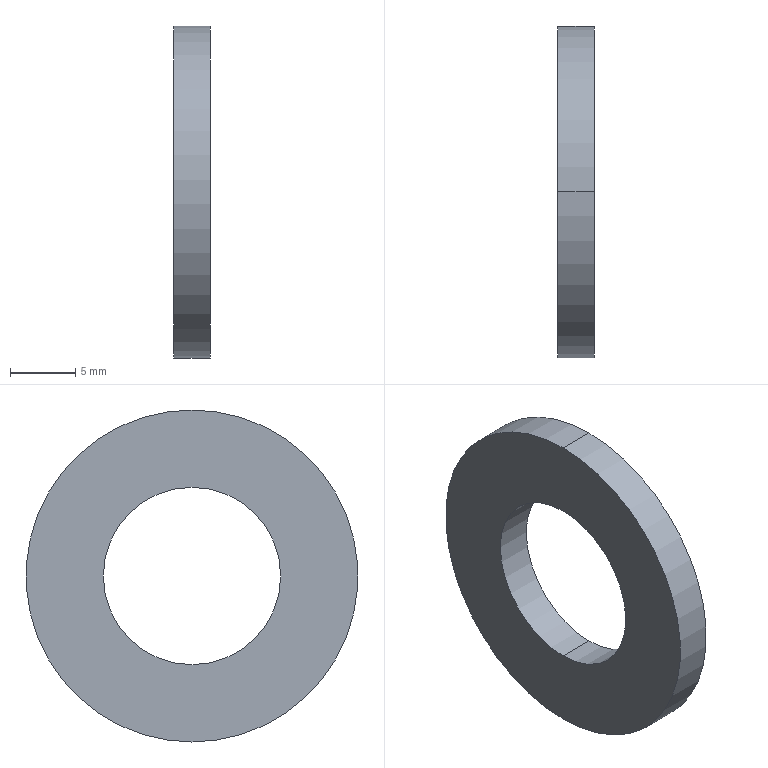Part | STEP file | flat washer narrow_am_B18.22M - Plain washer, 12 mm, narrow | 1 solid | 6 faces | box 2.8 x 25.4 x 25.4 mm | volume 1014 mm3 | cylinder 4 | plane 2 | commonest cylinder face diameters 13.57 x2 25.4 x2
STEP:
#1=CARTESIAN_POINT('',(0.,0.,0.));
#2=DIRECTION('',(0.,0.,1.));
#3=DIRECTION('',(1.,0.,0.));
#4=AXIS2_PLACEMENT_3D('',#1,#2,#3);
#5=CARTESIAN_POINT('',(0.,0.,12.7));
#6=VERTEX_POINT('',#5);
#7=CARTESIAN_POINT('',(0.,0.,-12.7));
#8=VERTEX_POINT('',#7);
#9=CARTESIAN_POINT('',(0.,0.,0.));
#10=DIRECTION('',(-1.,0.,0.));
#11=DIRECTION('',(0.,0.,1.));
#12=AXIS2_PLACEMENT_3D('',#9,#10,#11);
#13=CIRCLE('',#12,12.7);
#14=CARTESIAN_POINT('',(-34.925,0.,0.));
#15=DIRECTION('',(-1.,0.,0.));
#16=DIRECTION('',(0.,0.,1.));
#17=AXIS2_PLACEMENT_3D('',#14,#15,#16);
#18=CYLINDRICAL_SURFACE('',#17,12.7);
#19=CARTESIAN_POINT('',(0.,-34.925));
#20=DIRECTION('',(1.,0.));
#21=VECTOR('',#20,1.);
#22=LINE('',#19,#21);
#23=(GEOMETRIC_REPRESENTATION_CONTEXT(2)PARAMETRIC_REPRESENTATION_CONTEXT()REPRESENTATION_CONTEXT('',''));
#24=DEFINITIONAL_REPRESENTATION('',(#22),#23);
#25=PCURVE('',#18,#24);
#26=CARTESIAN_POINT('',(0.,6.785,0.));
#27=DIRECTION('',(-1.,0.,0.));
#28=DIRECTION('',(0.,0.,1.));
#29=AXIS2_PLACEMENT_3D('',#26,#27,#28);
#30=PLANE('',#29);
#31=CARTESIAN_POINT('',(0.,-6.785));
#32=DIRECTION('',(1.,0.));
#33=AXIS2_PLACEMENT_2D('',#31,#32);
#34=CIRCLE('',#33,12.7);
#35=(GEOMETRIC_REPRESENTATION_CONTEXT(2)PARAMETRIC_REPRESENTATION_CONTEXT()REPRESENTATION_CONTEXT('',''));
#36=DEFINITIONAL_REPRESENTATION('',(#34),#35);
#37=PCURVE('',#30,#36);
#38=SURFACE_CURVE('',#13,(#25,#37),.PCURVE_S1.);
#39=EDGE_CURVE('',#6,#8,#38,.T.);
#40=ORIENTED_EDGE('',*,*,#39,.T.);
#41=CARTESIAN_POINT('',(-2.8,0.,-12.7));
#42=VERTEX_POINT('',#41);
#43=CARTESIAN_POINT('',(-34.925,0.,-12.7));
#44=DIRECTION('',(-1.,0.,0.));
#45=VECTOR('',#44,1.);
#46=LINE('',#43,#45);
#47=CARTESIAN_POINT('',(3.142,0.));
#48=DIRECTION('',(0.,1.));
#49=VECTOR('',#48,1.);
#50=LINE('',#47,#49);
#51=(GEOMETRIC_REPRESENTATION_CONTEXT(2)PARAMETRIC_REPRESENTATION_CONTEXT()REPRESENTATION_CONTEXT('',''));
#52=DEFINITIONAL_REPRESENTATION('',(#50),#51);
#53=PCURVE('',#18,#52);
#54=CARTESIAN_POINT('',(-34.925,0.,0.));
#55=DIRECTION('',(-1.,0.,0.));
#56=DIRECTION('',(0.,0.,1.));
#57=AXIS2_PLACEMENT_3D('',#54,#55,#56);
#58=CYLINDRICAL_SURFACE('',#57,12.7);
#59=CARTESIAN_POINT('',(3.142,0.));
#60=DIRECTION('',(0.,1.));
#61=VECTOR('',#60,1.);
#62=LINE('',#59,#61);
#63=(GEOMETRIC_REPRESENTATION_CONTEXT(2)PARAMETRIC_REPRESENTATION_CONTEXT()REPRESENTATION_CONTEXT('',''));
#64=DEFINITIONAL_REPRESENTATION('',(#62),#63);
#65=PCURVE('',#58,#64);
#66=SURFACE_CURVE('',#46,(#53,#65),.PCURVE_S1.);
#67=EDGE_CURVE('',#8,#42,#66,.T.);
#68=ORIENTED_EDGE('',*,*,#67,.T.);
#69=CARTESIAN_POINT('',(-2.8,0.,12.7));
#70=VERTEX_POINT('',#69);
#71=CARTESIAN_POINT('',(-2.8,0.,0.));
#72=DIRECTION('',(-1.,0.,0.));
#73=DIRECTION('',(0.,0.,1.));
#74=AXIS2_PLACEMENT_3D('',#71,#72,#73);
#75=CIRCLE('',#74,12.7);
#76=CARTESIAN_POINT('',(0.,-32.125));
#77=DIRECTION('',(1.,0.));
#78=VECTOR('',#77,1.);
#79=LINE('',#76,#78);
#80=(GEOMETRIC_REPRESENTATION_CONTEXT(2)PARAMETRIC_REPRESENTATION_CONTEXT()REPRESENTATION_CONTEXT('',''));
#81=DEFINITIONAL_REPRESENTATION('',(#79),#80);
#82=PCURVE('',#18,#81);
#83=CARTESIAN_POINT('',(-2.8,12.7,0.));
#84=DIRECTION('',(1.,0.,0.));
#85=DIRECTION('',(0.,0.,-1.));
#86=AXIS2_PLACEMENT_3D('',#83,#84,#85);
#87=PLANE('',#86);
#88=CARTESIAN_POINT('',(-12.7,-12.7));
#89=CARTESIAN_POINT('',(-12.7,9.297));
#90=CARTESIAN_POINT('',(6.35,-1.701));
#91=CARTESIAN_POINT('',(25.4,-12.7));
#92=CARTESIAN_POINT('',(6.35,-23.699));
#93=CARTESIAN_POINT('',(-12.7,-34.697));
#94=CARTESIAN_POINT('',(-12.7,-12.7));
#95=(BOUNDED_CURVE()B_SPLINE_CURVE(2,(#88,#89,#90,#91,#92,#93,#94),.UNSPECIFIED.,.T.,.F.)B_SPLINE_CURVE_WITH_KNOTS((1,2,2,2,2,1),(-2.094,0.,2.094,4.189,6.283,8.378),.UNSPECIFIED.)CURVE()GEOMETRIC_REPRESENTATION_ITEM()RATIONAL_B_SPLINE_CURVE((1.,0.5,1.,0.5,1.,0.5,1.))REPRESENTATION_ITEM(''));
#96=(GEOMETRIC_REPRESENTATION_CONTEXT(2)PARAMETRIC_REPRESENTATION_CONTEXT()REPRESENTATION_CONTEXT('',''));
#97=DEFINITIONAL_REPRESENTATION('',(#95),#96);
#98=PCURVE('',#87,#97);
#99=SURFACE_CURVE('',#75,(#82,#98),.PCURVE_S1.);
#100=EDGE_CURVE('',#70,#42,#99,.T.);
#101=ORIENTED_EDGE('',*,*,#100,.F.);
#102=CARTESIAN_POINT('',(-34.925,0.,12.7));
#103=DIRECTION('',(-1.,0.,0.));
#104=VECTOR('',#103,1.);
#105=LINE('',#102,#104);
#106=CARTESIAN_POINT('',(0.,0.));
#107=DIRECTION('',(0.,1.));
#108=VECTOR('',#107,1.);
#109=LINE('',#106,#108);
#110=(GEOMETRIC_REPRESENTATION_CONTEXT(2)PARAMETRIC_REPRESENTATION_CONTEXT()REPRESENTATION_CONTEXT('',''));
#111=DEFINITIONAL_REPRESENTATION('',(#109),#110);
#112=PCURVE('',#18,#111);
#113=CARTESIAN_POINT('',(6.283,0.));
#114=DIRECTION('',(0.,1.));
#115=VECTOR('',#114,1.);
#116=LINE('',#113,#115);
#117=(GEOMETRIC_REPRESENTATION_CONTEXT(2)PARAMETRIC_REPRESENTATION_CONTEXT()REPRESENTATION_CONTEXT('',''));
#118=DEFINITIONAL_REPRESENTATION('',(#116),#117);
#119=PCURVE('',#58,#118);
#120=SURFACE_CURVE('',#105,(#112,#119),.PCURVE_S1.);
#121=EDGE_CURVE('',#6,#70,#120,.T.);
#122=ORIENTED_EDGE('',*,*,#121,.F.);
#123=EDGE_LOOP('',(#40,#68,#101,#122));
#124=FACE_BOUND('',#123,.T.);
#125=ADVANCED_FACE('',(#124),#18,.T.);
#126=CARTESIAN_POINT('',(0.,0.,6.785));
#127=VERTEX_POINT('',#126);
#128=CARTESIAN_POINT('',(-2.8,0.,6.785));
#129=VERTEX_POINT('',#128);
#130=CARTESIAN_POINT('',(-34.925,0.,6.785));
#131=DIRECTION('',(-1.,0.,0.));
#132=VECTOR('',#131,1.);
#133=LINE('',#130,#132);
#134=CARTESIAN_POINT('',(-34.925,0.,0.));
#135=DIRECTION('',(-1.,0.,0.));
#136=DIRECTION('',(0.,0.,1.));
#137=AXIS2_PLACEMENT_3D('',#134,#135,#136);
#138=CYLINDRICAL_SURFACE('',#137,6.785);
#139=CARTESIAN_POINT('',(6.283,0.));
#140=DIRECTION('',(0.,1.));
#141=VECTOR('',#140,1.);
#142=LINE('',#139,#141);
#143=(GEOMETRIC_REPRESENTATION_CONTEXT(2)PARAMETRIC_REPRESENTATION_CONTEXT()REPRESENTATION_CONTEXT('',''));
#144=DEFINITIONAL_REPRESENTATION('',(#142),#143);
#145=PCURVE('',#138,#144);
#146=CARTESIAN_POINT('',(-34.925,0.,0.));
#147=DIRECTION('',(-1.,0.,0.));
#148=DIRECTION('',(0.,0.,1.));
#149=AXIS2_PLACEMENT_3D('',#146,#147,#148);
#150=CYLINDRICAL_SURFACE('',#149,6.785);
#151=CARTESIAN_POINT('',(0.,0.));
#152=DIRECTION('',(0.,1.));
#153=VECTOR('',#152,1.);
#154=LINE('',#151,#153);
#155=(GEOMETRIC_REPRESENTATION_CONTEXT(2)PARAMETRIC_REPRESENTATION_CONTEXT()REPRESENTATION_CONTEXT('',''));
#156=DEFINITIONAL_REPRESENTATION('',(#154),#155);
#157=PCURVE('',#150,#156);
#158=SURFACE_CURVE('',#133,(#145,#157),.PCURVE_S1.);
#159=EDGE_CURVE('',#127,#129,#158,.T.);
#160=ORIENTED_EDGE('',*,*,#159,.T.);
#161=CARTESIAN_POINT('',(-2.8,0.,-6.785));
#162=VERTEX_POINT('',#161);
#163=CARTESIAN_POINT('',(-2.8,0.,0.));
#164=DIRECTION('',(-1.,0.,0.));
#165=DIRECTION('',(0.,0.,1.));
#166=AXIS2_PLACEMENT_3D('',#163,#164,#165);
#167=CIRCLE('',#166,6.785);
#168=CARTESIAN_POINT('',(0.,-32.125));
#169=DIRECTION('',(1.,0.));
#170=VECTOR('',#169,1.);
#171=LINE('',#168,#170);
#172=(GEOMETRIC_REPRESENTATION_CONTEXT(2)PARAMETRIC_REPRESENTATION_CONTEXT()REPRESENTATION_CONTEXT('',''));
#173=DEFINITIONAL_REPRESENTATION('',(#171),#172);
#174=PCURVE('',#138,#173);
#175=CARTESIAN_POINT('',(-6.785,-12.7));
#176=CARTESIAN_POINT('',(-6.785,-0.948));
#177=CARTESIAN_POINT('',(3.393,-6.824));
#178=CARTESIAN_POINT('',(13.57,-12.7));
#179=CARTESIAN_POINT('',(3.393,-18.576));
#180=CARTESIAN_POINT('',(-6.785,-24.452));
#181=CARTESIAN_POINT('',(-6.785,-12.7));
#182=(BOUNDED_CURVE()B_SPLINE_CURVE(2,(#175,#176,#177,#178,#179,#180,#181),.UNSPECIFIED.,.T.,.F.)B_SPLINE_CURVE_WITH_KNOTS((1,2,2,2,2,1),(-2.094,0.,2.094,4.189,6.283,8.378),.UNSPECIFIED.)CURVE()GEOMETRIC_REPRESENTATION_ITEM()RATIONAL_B_SPLINE_CURVE((1.,0.5,1.,0.5,1.,0.5,1.))REPRESENTATION_ITEM(''));
#183=(GEOMETRIC_REPRESENTATION_CONTEXT(2)PARAMETRIC_REPRESENTATION_CONTEXT()REPRESENTATION_CONTEXT('',''));
#184=DEFINITIONAL_REPRESENTATION('',(#182),#183);
#185=PCURVE('',#87,#184);
#186=SURFACE_CURVE('',#167,(#174,#185),.PCURVE_S1.);
#187=EDGE_CURVE('',#162,#129,#186,.T.);
#188=ORIENTED_EDGE('',*,*,#187,.F.);
#189=CARTESIAN_POINT('',(0.,0.,-6.785));
#190=VERTEX_POINT('',#189);
#191=CARTESIAN_POINT('',(-34.925,0.,-6.785));
#192=DIRECTION('',(-1.,0.,0.));
#193=VECTOR('',#192,1.);
#194=LINE('',#191,#193);
#195=CARTESIAN_POINT('',(3.142,0.));
#196=DIRECTION('',(0.,1.));
#197=VECTOR('',#196,1.);
#198=LINE('',#195,#197);
#199=(GEOMETRIC_REPRESENTATION_CONTEXT(2)PARAMETRIC_REPRESENTATION_CONTEXT()REPRESENTATION_CONTEXT('',''));
#200=DEFINITIONAL_REPRESENTATION('',(#198),#199);
#201=PCURVE('',#138,#200);
#202=CARTESIAN_POINT('',(3.142,0.));
#203=DIRECTION('',(0.,1.));
#204=VECTOR('',#203,1.);
#205=LINE('',#202,#204);
#206=(GEOMETRIC_REPRESENTATION_CONTEXT(2)PARAMETRIC_REPRESENTATION_CONTEXT()REPRESENTATION_CONTEXT('',''));
#207=DEFINITIONAL_REPRESENTATION('',(#205),#206);
#208=PCURVE('',#150,#207);
#209=SURFACE_CURVE('',#194,(#201,#208),.PCURVE_S1.);
#210=EDGE_CURVE('',#190,#162,#209,.T.);
#211=ORIENTED_EDGE('',*,*,#210,.F.);
#212=CARTESIAN_POINT('',(0.,0.,0.));
#213=DIRECTION('',(-1.,0.,0.));
#214=DIRECTION('',(0.,0.,1.));
#215=AXIS2_PLACEMENT_3D('',#212,#213,#214);
#216=CIRCLE('',#215,6.785);
#217=CARTESIAN_POINT('',(0.,-34.925));
#218=DIRECTION('',(1.,0.));
#219=VECTOR('',#218,1.);
#220=LINE('',#217,#219);
#221=(GEOMETRIC_REPRESENTATION_CONTEXT(2)PARAMETRIC_REPRESENTATION_CONTEXT()REPRESENTATION_CONTEXT('',''));
#222=DEFINITIONAL_REPRESENTATION('',(#220),#221);
#223=PCURVE('',#138,#222);
#224=CARTESIAN_POINT('',(0.,-6.785));
#225=DIRECTION('',(1.,0.));
#226=AXIS2_PLACEMENT_2D('',#224,#225);
#227=CIRCLE('',#226,6.785);
#228=(GEOMETRIC_REPRESENTATION_CONTEXT(2)PARAMETRIC_REPRESENTATION_CONTEXT()REPRESENTATION_CONTEXT('',''));
#229=DEFINITIONAL_REPRESENTATION('',(#227),#228);
#230=PCURVE('',#30,#229);
#231=SURFACE_CURVE('',#216,(#223,#230),.PCURVE_S1.);
#232=EDGE_CURVE('',#190,#127,#231,.T.);
#233=ORIENTED_EDGE('',*,*,#232,.T.);
#234=EDGE_LOOP('',(#160,#188,#211,#233));
#235=FACE_BOUND('',#234,.F.);
#236=ADVANCED_FACE('',(#235),#138,.F.);
#237=CARTESIAN_POINT('',(-2.8,0.,0.));
#238=DIRECTION('',(-1.,0.,0.));
#239=DIRECTION('',(0.,0.,1.));
#240=AXIS2_PLACEMENT_3D('',#237,#238,#239);
#241=CIRCLE('',#240,6.785);
#242=CARTESIAN_POINT('',(0.,-32.125));
#243=DIRECTION('',(1.,0.));
#244=VECTOR('',#243,1.);
#245=LINE('',#242,#244);
#246=(GEOMETRIC_REPRESENTATION_CONTEXT(2)PARAMETRIC_REPRESENTATION_CONTEXT()REPRESENTATION_CONTEXT('',''));
#247=DEFINITIONAL_REPRESENTATION('',(#245),#246);
#248=PCURVE('',#150,#247);
#249=CARTESIAN_POINT('',(-6.785,-12.7));
#250=CARTESIAN_POINT('',(-6.785,-0.948));
#251=CARTESIAN_POINT('',(3.393,-6.824));
#252=CARTESIAN_POINT('',(13.57,-12.7));
#253=CARTESIAN_POINT('',(3.393,-18.576));
#254=CARTESIAN_POINT('',(-6.785,-24.452));
#255=CARTESIAN_POINT('',(-6.785,-12.7));
#256=(BOUNDED_CURVE()B_SPLINE_CURVE(2,(#249,#250,#251,#252,#253,#254,#255),.UNSPECIFIED.,.T.,.F.)B_SPLINE_CURVE_WITH_KNOTS((1,2,2,2,2,1),(-2.094,0.,2.094,4.189,6.283,8.378),.UNSPECIFIED.)CURVE()GEOMETRIC_REPRESENTATION_ITEM()RATIONAL_B_SPLINE_CURVE((1.,0.5,1.,0.5,1.,0.5,1.))REPRESENTATION_ITEM(''));
#257=(GEOMETRIC_REPRESENTATION_CONTEXT(2)PARAMETRIC_REPRESENTATION_CONTEXT()REPRESENTATION_CONTEXT('',''));
#258=DEFINITIONAL_REPRESENTATION('',(#256),#257);
#259=PCURVE('',#87,#258);
#260=SURFACE_CURVE('',#241,(#248,#259),.PCURVE_S1.);
#261=EDGE_CURVE('',#129,#162,#260,.T.);
#262=ORIENTED_EDGE('',*,*,#261,.F.);
#263=ORIENTED_EDGE('',*,*,#159,.F.);
#264=CARTESIAN_POINT('',(0.,0.,0.));
#265=DIRECTION('',(-1.,0.,0.));
#266=DIRECTION('',(0.,0.,1.));
#267=AXIS2_PLACEMENT_3D('',#264,#265,#266);
#268=CIRCLE('',#267,6.785);
#269=CARTESIAN_POINT('',(0.,-34.925));
#270=DIRECTION('',(1.,0.));
#271=VECTOR('',#270,1.);
#272=LINE('',#269,#271);
#273=(GEOMETRIC_REPRESENTATION_CONTEXT(2)PARAMETRIC_REPRESENTATION_CONTEXT()REPRESENTATION_CONTEXT('',''));
#274=DEFINITIONAL_REPRESENTATION('',(#272),#273);
#275=PCURVE('',#150,#274);
#276=CARTESIAN_POINT('',(0.,-6.785));
#277=DIRECTION('',(1.,0.));
#278=AXIS2_PLACEMENT_2D('',#276,#277);
#279=CIRCLE('',#278,6.785);
#280=(GEOMETRIC_REPRESENTATION_CONTEXT(2)PARAMETRIC_REPRESENTATION_CONTEXT()REPRESENTATION_CONTEXT('',''));
#281=DEFINITIONAL_REPRESENTATION('',(#279),#280);
#282=PCURVE('',#30,#281);
#283=SURFACE_CURVE('',#268,(#275,#282),.PCURVE_S1.);
#284=EDGE_CURVE('',#127,#190,#283,.T.);
#285=ORIENTED_EDGE('',*,*,#284,.T.);
#286=ORIENTED_EDGE('',*,*,#210,.T.);
#287=EDGE_LOOP('',(#262,#263,#285,#286));
#288=FACE_BOUND('',#287,.F.);
#289=ADVANCED_FACE('',(#288),#150,.F.);
#290=ORIENTED_EDGE('',*,*,#39,.F.);
#291=CARTESIAN_POINT('',(0.,0.,0.));
#292=DIRECTION('',(-1.,0.,0.));
#293=DIRECTION('',(0.,0.,1.));
#294=AXIS2_PLACEMENT_3D('',#291,#292,#293);
#295=CIRCLE('',#294,12.7);
#296=CARTESIAN_POINT('',(0.,-6.785));
#297=DIRECTION('',(1.,0.));
#298=AXIS2_PLACEMENT_2D('',#296,#297);
#299=CIRCLE('',#298,12.7);
#300=(GEOMETRIC_REPRESENTATION_CONTEXT(2)PARAMETRIC_REPRESENTATION_CONTEXT()REPRESENTATION_CONTEXT('',''));
#301=DEFINITIONAL_REPRESENTATION('',(#299),#300);
#302=PCURVE('',#30,#301);
#303=CARTESIAN_POINT('',(0.,-34.925));
#304=DIRECTION('',(1.,0.));
#305=VECTOR('',#304,1.);
#306=LINE('',#303,#305);
#307=(GEOMETRIC_REPRESENTATION_CONTEXT(2)PARAMETRIC_REPRESENTATION_CONTEXT()REPRESENTATION_CONTEXT('',''));
#308=DEFINITIONAL_REPRESENTATION('',(#306),#307);
#309=PCURVE('',#58,#308);
#310=SURFACE_CURVE('',#295,(#302,#309),.PCURVE_S1.);
#311=EDGE_CURVE('',#8,#6,#310,.T.);
#312=ORIENTED_EDGE('',*,*,#311,.F.);
#313=EDGE_LOOP('',(#290,#312));
#314=FACE_BOUND('',#313,.T.);
#315=ORIENTED_EDGE('',*,*,#284,.T.);
#316=ORIENTED_EDGE('',*,*,#232,.T.);
#317=EDGE_LOOP('',(#315,#316));
#318=FACE_BOUND('',#317,.T.);
#319=ADVANCED_FACE('',(#314,#318),#30,.F.);
#320=ORIENTED_EDGE('',*,*,#67,.F.);
#321=ORIENTED_EDGE('',*,*,#311,.T.);
#322=ORIENTED_EDGE('',*,*,#121,.T.);
#323=CARTESIAN_POINT('',(-2.8,0.,0.));
#324=DIRECTION('',(-1.,0.,0.));
#325=DIRECTION('',(0.,0.,1.));
#326=AXIS2_PLACEMENT_3D('',#323,#324,#325);
#327=CIRCLE('',#326,12.7);
#328=CARTESIAN_POINT('',(0.,-32.125));
#329=DIRECTION('',(1.,0.));
#330=VECTOR('',#329,1.);
#331=LINE('',#328,#330);
#332=(GEOMETRIC_REPRESENTATION_CONTEXT(2)PARAMETRIC_REPRESENTATION_CONTEXT()REPRESENTATION_CONTEXT('',''));
#333=DEFINITIONAL_REPRESENTATION('',(#331),#332);
#334=PCURVE('',#58,#333);
#335=CARTESIAN_POINT('',(-12.7,-12.7));
#336=CARTESIAN_POINT('',(-12.7,9.297));
#337=CARTESIAN_POINT('',(6.35,-1.701));
#338=CARTESIAN_POINT('',(25.4,-12.7));
#339=CARTESIAN_POINT('',(6.35,-23.699));
#340=CARTESIAN_POINT('',(-12.7,-34.697));
#341=CARTESIAN_POINT('',(-12.7,-12.7));
#342=(BOUNDED_CURVE()B_SPLINE_CURVE(2,(#335,#336,#337,#338,#339,#340,#341),.UNSPECIFIED.,.T.,.F.)B_SPLINE_CURVE_WITH_KNOTS((1,2,2,2,2,1),(-2.094,0.,2.094,4.189,6.283,8.378),.UNSPECIFIED.)CURVE()GEOMETRIC_REPRESENTATION_ITEM()RATIONAL_B_SPLINE_CURVE((1.,0.5,1.,0.5,1.,0.5,1.))REPRESENTATION_ITEM(''));
#343=(GEOMETRIC_REPRESENTATION_CONTEXT(2)PARAMETRIC_REPRESENTATION_CONTEXT()REPRESENTATION_CONTEXT('',''));
#344=DEFINITIONAL_REPRESENTATION('',(#342),#343);
#345=PCURVE('',#87,#344);
#346=SURFACE_CURVE('',#327,(#334,#345),.PCURVE_S1.);
#347=EDGE_CURVE('',#42,#70,#346,.T.);
#348=ORIENTED_EDGE('',*,*,#347,.F.);
#349=EDGE_LOOP('',(#320,#321,#322,#348));
#350=FACE_BOUND('',#349,.T.);
#351=ADVANCED_FACE('',(#350),#58,.T.);
#352=ORIENTED_EDGE('',*,*,#261,.F.);
#353=ORIENTED_EDGE('',*,*,#187,.F.);
#354=EDGE_LOOP('',(#352,#353));
#355=FACE_BOUND('',#354,.T.);
#356=ORIENTED_EDGE('',*,*,#100,.T.);
#357=ORIENTED_EDGE('',*,*,#347,.T.);
#358=EDGE_LOOP('',(#356,#357));
#359=FACE_BOUND('',#358,.T.);
#360=ADVANCED_FACE('',(#355,#359),#87,.F.);
#361=CLOSED_SHELL('',(#125,#236,#289,#319,#351,#360));
#362=MANIFOLD_SOLID_BREP('',#361);
#363=(LENGTH_UNIT()NAMED_UNIT(*)SI_UNIT(.MILLI.,.METRE.));
#364=UNCERTAINTY_MEASURE_WITH_UNIT(LENGTH_MEASURE(0.0000001),#363,'','');
#365=(NAMED_UNIT(*)PLANE_ANGLE_UNIT()SI_UNIT($,.RADIAN.));
#366=(NAMED_UNIT(*)SI_UNIT($,.STERADIAN.)SOLID_ANGLE_UNIT());
#367=(GEOMETRIC_REPRESENTATION_CONTEXT(3)GLOBAL_UNCERTAINTY_ASSIGNED_CONTEXT((#364))GLOBAL_UNIT_ASSIGNED_CONTEXT((#363,#365,#366))REPRESENTATION_CONTEXT('',''));
#368=ADVANCED_BREP_SHAPE_REPRESENTATION('',(#4,#362),#367);